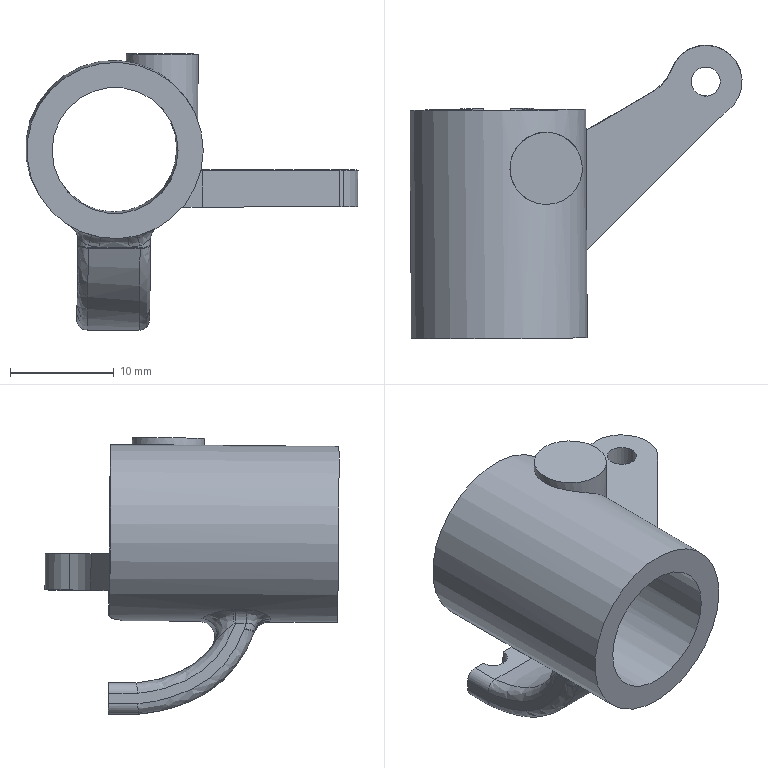Part | STEP file | Zaokr_glenie5_1 | 1 solid | 58 faces | box 32.058 x 28.351 x 26.679 mm | volume 3338 mm3 | spline 23 | cylinder 19 | plane 16 | commonest cylinder face diameters 2 x6 2.7 x2 3 x2 4 x2 7.98 x2 2.8 x1